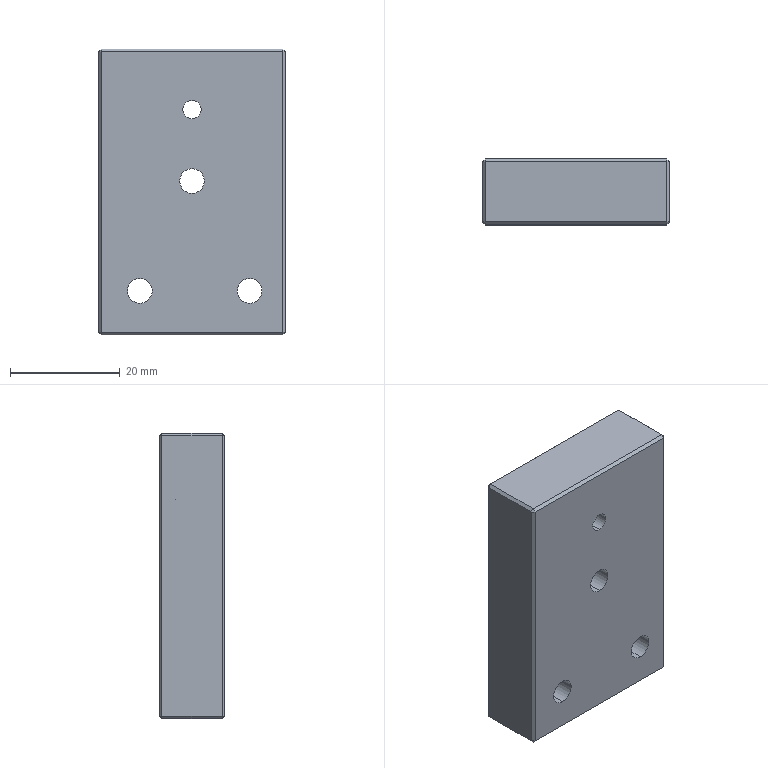Part | STEP file | ND25021-01-JDKM-58-TL | 1 solid | 43 faces | box 34 x 12 x 52 mm | volume 20039 mm3 | plane 29 | cylinder 14 | commonest cylinder face diameters 4.5 x6 8 x6 3.3 x2